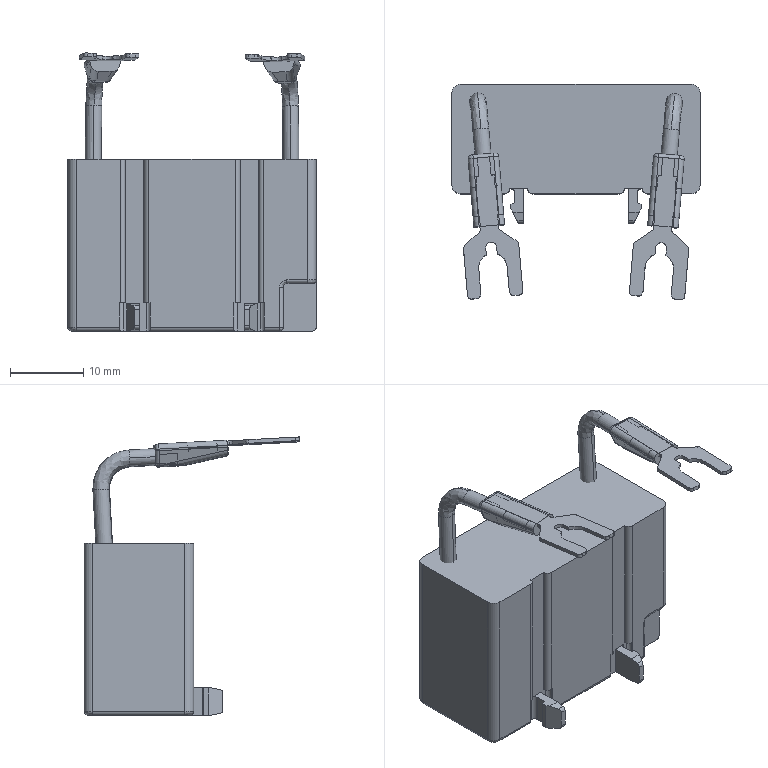Part | SolidWorks | features BaseBody 7 | 7 solids | 344 faces | box 34 x 29.543 x 38.064 mm | volume 10047 mm3 | plane 179 | cylinder 138 | spline 19 | torus 8 | commonest cylinder face diameters 1 x67 1.4 x22 2 x9 0.4 x8 0.6 x8 2.2 x8